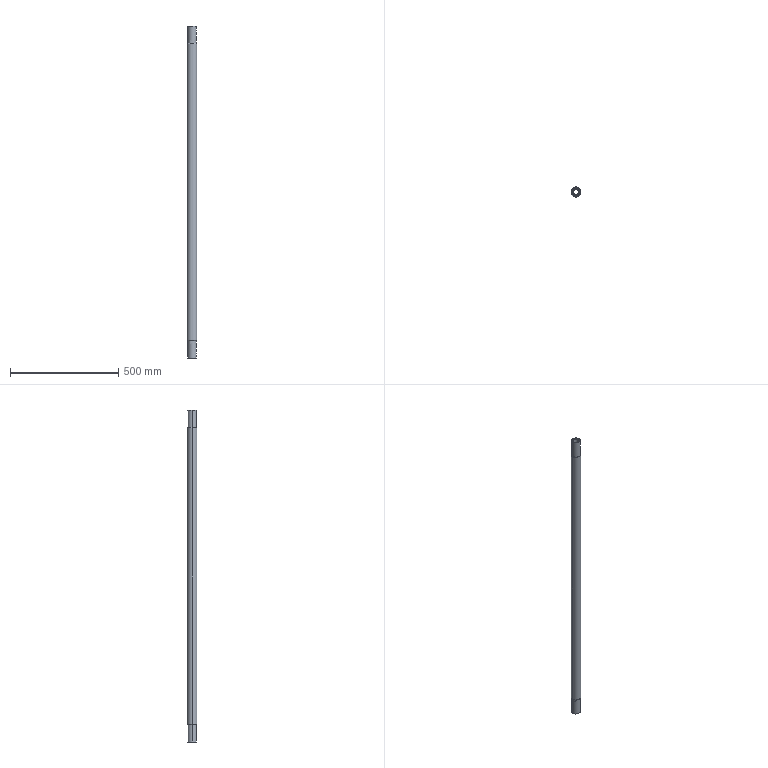Part | SolidWorks | features ICE 5, HoleWzd 2, MirrorPattern 2, Chamfer 1, Extrusion 1 | 1 solid | 46 faces | box 45 x 45 x 1535 mm | volume 1600076 mm3 | cylinder 27 | plane 12 | cone 7 | commonest cylinder face diameters 12 x8 26.5 x4 32 x4 40 x4 6 x3 25 x2